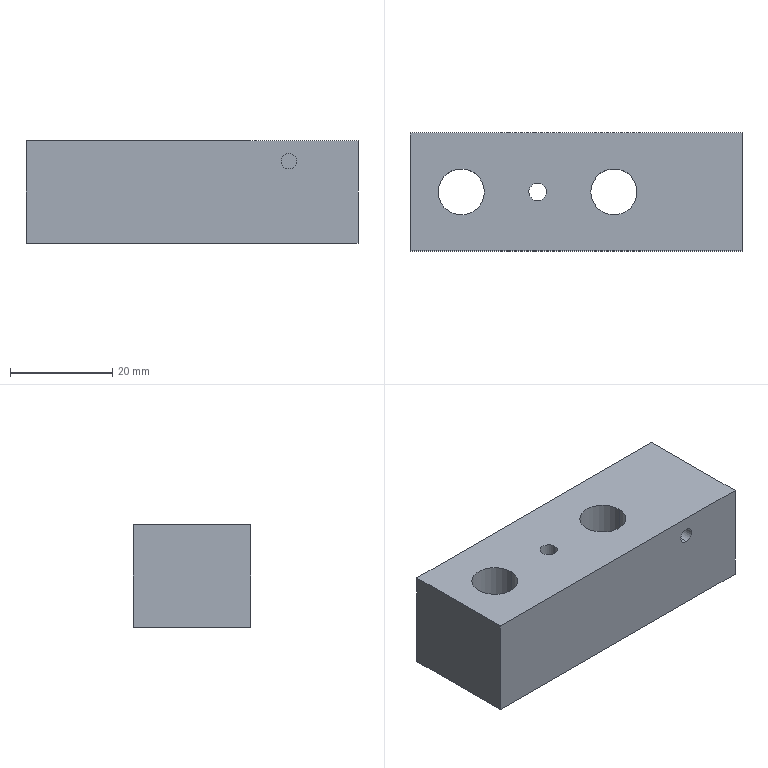Part | SolidWorks | features 3DProfileFeature 2, HoleWzd 2, Extrusion 1, ICE 1 | 1 solid | 24 faces | box 64.8 x 23 x 20 mm | volume 24913 mm3 | cylinder 14 | plane 10 | commonest cylinder face diameters 9 x4 15 x4 3 x2 3.4 x2 6.5 x2
STEP:
#1=CARTESIAN_POINT('',(-4.25,11.5,-6.6));
#2=VERTEX_POINT('',#1);
#3=CARTESIAN_POINT('',(-10.75,11.5,-6.6));
#4=VERTEX_POINT('',#3);
#5=CARTESIAN_POINT('',(-7.5,11.5,-6.6));
#6=DIRECTION('',(0.,0.,-1.));
#7=DIRECTION('',(-1.,0.,0.));
#8=AXIS2_PLACEMENT_3D('',#5,#6,#7);
#9=CIRCLE('',#8,3.25);
#10=EDGE_CURVE('',#2,#4,#9,.T.);
#11=ORIENTED_EDGE('',*,*,#10,.F.);
#12=CARTESIAN_POINT('',(-4.25,11.5,-10.));
#13=VERTEX_POINT('',#12);
#14=CARTESIAN_POINT('',(-4.25,11.5,-10.));
#15=DIRECTION('',(0.,0.,-1.));
#16=VECTOR('',#15,1000.);
#17=LINE('',#14,#16);
#18=EDGE_CURVE('',#2,#13,#17,.T.);
#19=ORIENTED_EDGE('',*,*,#18,.T.);
#20=CARTESIAN_POINT('',(-10.75,11.5,-10.));
#21=VERTEX_POINT('',#20);
#22=CARTESIAN_POINT('',(-7.5,11.5,-10.));
#23=DIRECTION('',(0.,0.,-1.));
#24=DIRECTION('',(-1.,0.,0.));
#25=AXIS2_PLACEMENT_3D('',#22,#23,#24);
#26=CIRCLE('',#25,3.25);
#27=EDGE_CURVE('',#13,#21,#26,.T.);
#28=ORIENTED_EDGE('',*,*,#27,.T.);
#29=CARTESIAN_POINT('',(-10.75,11.5,-10.));
#30=DIRECTION('',(0.,0.,-1.));
#31=VECTOR('',#30,1000.);
#32=LINE('',#29,#31);
#33=EDGE_CURVE('',#4,#21,#32,.T.);
#34=ORIENTED_EDGE('',*,*,#33,.F.);
#35=EDGE_LOOP('',(#11,#19,#28,#34));
#36=FACE_OUTER_BOUND('',#35,.T.);
#37=CARTESIAN_POINT('',(-7.5,11.5,-10.));
#38=DIRECTION('',(0.,0.,-1.));
#39=DIRECTION('',(-1.,0.,0.));
#40=AXIS2_PLACEMENT_3D('',#37,#38,#39);
#41=CYLINDRICAL_SURFACE('',#40,3.25);
#42=ADVANCED_FACE('',(#36),#41,.F.);
#43=CARTESIAN_POINT('',(-5.8,11.5,10.));
#44=VERTEX_POINT('',#43);
#45=CARTESIAN_POINT('',(-9.2,11.5,10.));
#46=VERTEX_POINT('',#45);
#47=CARTESIAN_POINT('',(-7.5,11.5,10.));
#48=DIRECTION('',(0.,0.,-1.));
#49=DIRECTION('',(-1.,0.,0.));
#50=AXIS2_PLACEMENT_3D('',#47,#48,#49);
#51=CIRCLE('',#50,1.7);
#52=EDGE_CURVE('',#44,#46,#51,.T.);
#53=ORIENTED_EDGE('',*,*,#52,.F.);
#54=CARTESIAN_POINT('',(-5.8,11.5,-6.6));
#55=VERTEX_POINT('',#54);
#56=CARTESIAN_POINT('',(-5.8,11.5,-10.));
#57=DIRECTION('',(0.,0.,-1.));
#58=VECTOR('',#57,1000.);
#59=LINE('',#56,#58);
#60=EDGE_CURVE('',#44,#55,#59,.T.);
#61=ORIENTED_EDGE('',*,*,#60,.T.);
#62=CARTESIAN_POINT('',(-9.2,11.5,-6.6));
#63=VERTEX_POINT('',#62);
#64=CARTESIAN_POINT('',(-7.5,11.5,-6.6));
#65=DIRECTION('',(0.,0.,-1.));
#66=DIRECTION('',(-1.,0.,0.));
#67=AXIS2_PLACEMENT_3D('',#64,#65,#66);
#68=CIRCLE('',#67,1.7);
#69=EDGE_CURVE('',#55,#63,#68,.T.);
#70=ORIENTED_EDGE('',*,*,#69,.T.);
#71=CARTESIAN_POINT('',(-9.2,11.5,-10.));
#72=DIRECTION('',(0.,0.,-1.));
#73=VECTOR('',#72,1000.);
#74=LINE('',#71,#73);
#75=EDGE_CURVE('',#46,#63,#74,.T.);
#76=ORIENTED_EDGE('',*,*,#75,.F.);
#77=EDGE_LOOP('',(#53,#61,#70,#76));
#78=FACE_OUTER_BOUND('',#77,.T.);
#79=CARTESIAN_POINT('',(-7.5,11.5,-10.));
#80=DIRECTION('',(0.,0.,-1.));
#81=DIRECTION('',(-1.,0.,0.));
#82=AXIS2_PLACEMENT_3D('',#79,#80,#81);
#83=CYLINDRICAL_SURFACE('',#82,1.7);
#84=ADVANCED_FACE('',(#78),#83,.F.);
#85=CARTESIAN_POINT('',(-14.9,11.5,-1.4));
#86=VERTEX_POINT('',#85);
#87=CARTESIAN_POINT('',(-29.9,11.5,-1.4));
#88=VERTEX_POINT('',#87);
#89=CARTESIAN_POINT('',(-22.4,11.5,-1.4));
#90=DIRECTION('',(0.,0.,-1.));
#91=DIRECTION('',(-1.,0.,0.));
#92=AXIS2_PLACEMENT_3D('',#89,#90,#91);
#93=CIRCLE('',#92,7.5);
#94=EDGE_CURVE('',#86,#88,#93,.T.);
#95=ORIENTED_EDGE('',*,*,#94,.F.);
#96=CARTESIAN_POINT('',(-14.9,11.5,-10.));
#97=VERTEX_POINT('',#96);
#98=CARTESIAN_POINT('',(-14.9,11.5,-10.));
#99=DIRECTION('',(0.,0.,-1.));
#100=VECTOR('',#99,1000.);
#101=LINE('',#98,#100);
#102=EDGE_CURVE('',#86,#97,#101,.T.);
#103=ORIENTED_EDGE('',*,*,#102,.T.);
#104=CARTESIAN_POINT('',(-29.9,11.5,-10.));
#105=VERTEX_POINT('',#104);
#106=CARTESIAN_POINT('',(-22.4,11.5,-10.));
#107=DIRECTION('',(0.,0.,-1.));
#108=DIRECTION('',(-1.,0.,0.));
#109=AXIS2_PLACEMENT_3D('',#106,#107,#108);
#110=CIRCLE('',#109,7.5);
#111=EDGE_CURVE('',#97,#105,#110,.T.);
#112=ORIENTED_EDGE('',*,*,#111,.T.);
#113=CARTESIAN_POINT('',(-29.9,11.5,-10.));
#114=DIRECTION('',(0.,0.,-1.));
#115=VECTOR('',#114,1000.);
#116=LINE('',#113,#115);
#117=EDGE_CURVE('',#88,#105,#116,.T.);
#118=ORIENTED_EDGE('',*,*,#117,.F.);
#119=EDGE_LOOP('',(#95,#103,#112,#118));
#120=FACE_OUTER_BOUND('',#119,.T.);
#121=CARTESIAN_POINT('',(-22.4,11.5,-10.));
#122=DIRECTION('',(0.,0.,-1.));
#123=DIRECTION('',(-1.,0.,0.));
#124=AXIS2_PLACEMENT_3D('',#121,#122,#123);
#125=CYLINDRICAL_SURFACE('',#124,7.5);
#126=ADVANCED_FACE('',(#120),#125,.F.);
#127=CARTESIAN_POINT('',(-17.9,11.5,10.));
#128=VERTEX_POINT('',#127);
#129=CARTESIAN_POINT('',(-26.9,11.5,10.));
#130=VERTEX_POINT('',#129);
#131=CARTESIAN_POINT('',(-22.4,11.5,10.));
#132=DIRECTION('',(0.,0.,-1.));
#133=DIRECTION('',(-1.,0.,0.));
#134=AXIS2_PLACEMENT_3D('',#131,#132,#133);
#135=CIRCLE('',#134,4.5);
#136=EDGE_CURVE('',#128,#130,#135,.T.);
#137=ORIENTED_EDGE('',*,*,#136,.F.);
#138=CARTESIAN_POINT('',(-17.9,11.5,-1.4));
#139=VERTEX_POINT('',#138);
#140=CARTESIAN_POINT('',(-17.9,11.5,-10.));
#141=DIRECTION('',(0.,0.,-1.));
#142=VECTOR('',#141,1000.);
#143=LINE('',#140,#142);
#144=EDGE_CURVE('',#128,#139,#143,.T.);
#145=ORIENTED_EDGE('',*,*,#144,.T.);
#146=CARTESIAN_POINT('',(-26.9,11.5,-1.4));
#147=VERTEX_POINT('',#146);
#148=CARTESIAN_POINT('',(-22.4,11.5,-1.4));
#149=DIRECTION('',(0.,0.,-1.));
#150=DIRECTION('',(-1.,0.,0.));
#151=AXIS2_PLACEMENT_3D('',#148,#149,#150);
#152=CIRCLE('',#151,4.5);
#153=EDGE_CURVE('',#139,#147,#152,.T.);
#154=ORIENTED_EDGE('',*,*,#153,.T.);
#155=CARTESIAN_POINT('',(-26.9,11.5,-10.));
#156=DIRECTION('',(0.,0.,-1.));
#157=VECTOR('',#156,1000.);
#158=LINE('',#155,#157);
#159=EDGE_CURVE('',#130,#147,#158,.T.);
#160=ORIENTED_EDGE('',*,*,#159,.F.);
#161=EDGE_LOOP('',(#137,#145,#154,#160));
#162=FACE_OUTER_BOUND('',#161,.T.);
#163=CARTESIAN_POINT('',(-22.4,11.5,-10.));
#164=DIRECTION('',(0.,0.,-1.));
#165=DIRECTION('',(-1.,0.,0.));
#166=AXIS2_PLACEMENT_3D('',#163,#164,#165);
#167=CYLINDRICAL_SURFACE('',#166,4.5);
#168=ADVANCED_FACE('',(#162),#167,.F.);
#169=CARTESIAN_POINT('',(14.9,11.5,-1.4));
#170=VERTEX_POINT('',#169);
#171=CARTESIAN_POINT('',(-0.1,11.5,-1.4));
#172=VERTEX_POINT('',#171);
#173=CARTESIAN_POINT('',(7.4,11.5,-1.4));
#174=DIRECTION('',(0.,0.,-1.));
#175=DIRECTION('',(-1.,0.,0.));
#176=AXIS2_PLACEMENT_3D('',#173,#174,#175);
#177=CIRCLE('',#176,7.5);
#178=EDGE_CURVE('',#170,#172,#177,.T.);
#179=ORIENTED_EDGE('',*,*,#178,.F.);
#180=CARTESIAN_POINT('',(14.9,11.5,-10.));
#181=VERTEX_POINT('',#180);
#182=CARTESIAN_POINT('',(14.9,11.5,-10.));
#183=DIRECTION('',(0.,0.,-1.));
#184=VECTOR('',#183,1000.);
#185=LINE('',#182,#184);
#186=EDGE_CURVE('',#170,#181,#185,.T.);
#187=ORIENTED_EDGE('',*,*,#186,.T.);
#188=CARTESIAN_POINT('',(-0.1,11.5,-10.));
#189=VERTEX_POINT('',#188);
#190=CARTESIAN_POINT('',(7.4,11.5,-10.));
#191=DIRECTION('',(0.,0.,-1.));
#192=DIRECTION('',(-1.,0.,0.));
#193=AXIS2_PLACEMENT_3D('',#190,#191,#192);
#194=CIRCLE('',#193,7.5);
#195=EDGE_CURVE('',#181,#189,#194,.T.);
#196=ORIENTED_EDGE('',*,*,#195,.T.);
#197=CARTESIAN_POINT('',(-0.1,11.5,-10.));
#198=DIRECTION('',(0.,0.,-1.));
#199=VECTOR('',#198,1000.);
#200=LINE('',#197,#199);
#201=EDGE_CURVE('',#172,#189,#200,.T.);
#202=ORIENTED_EDGE('',*,*,#201,.F.);
#203=EDGE_LOOP('',(#179,#187,#196,#202));
#204=FACE_OUTER_BOUND('',#203,.T.);
#205=CARTESIAN_POINT('',(7.4,11.5,-10.));
#206=DIRECTION('',(0.,0.,-1.));
#207=DIRECTION('',(-1.,0.,0.));
#208=AXIS2_PLACEMENT_3D('',#205,#206,#207);
#209=CYLINDRICAL_SURFACE('',#208,7.5);
#210=ADVANCED_FACE('',(#204),#209,.F.);
#211=CARTESIAN_POINT('',(11.9,11.5,10.));
#212=VERTEX_POINT('',#211);
#213=CARTESIAN_POINT('',(2.9,11.5,10.));
#214=VERTEX_POINT('',#213);
#215=CARTESIAN_POINT('',(7.4,11.5,10.));
#216=DIRECTION('',(0.,0.,-1.));
#217=DIRECTION('',(-1.,0.,0.));
#218=AXIS2_PLACEMENT_3D('',#215,#216,#217);
#219=CIRCLE('',#218,4.5);
#220=EDGE_CURVE('',#212,#214,#219,.T.);
#221=ORIENTED_EDGE('',*,*,#220,.F.);
#222=CARTESIAN_POINT('',(11.9,11.5,-1.4));
#223=VERTEX_POINT('',#222);
#224=CARTESIAN_POINT('',(11.9,11.5,-10.));
#225=DIRECTION('',(0.,0.,-1.));
#226=VECTOR('',#225,1000.);
#227=LINE('',#224,#226);
#228=EDGE_CURVE('',#212,#223,#227,.T.);
#229=ORIENTED_EDGE('',*,*,#228,.T.);
#230=CARTESIAN_POINT('',(2.9,11.5,-1.4));
#231=VERTEX_POINT('',#230);
#232=CARTESIAN_POINT('',(7.4,11.5,-1.4));
#233=DIRECTION('',(0.,0.,-1.));
#234=DIRECTION('',(-1.,0.,0.));
#235=AXIS2_PLACEMENT_3D('',#232,#233,#234);
#236=CIRCLE('',#235,4.5);
#237=EDGE_CURVE('',#223,#231,#236,.T.);
#238=ORIENTED_EDGE('',*,*,#237,.T.);
#239=CARTESIAN_POINT('',(2.9,11.5,-10.));
#240=DIRECTION('',(0.,0.,-1.));
#241=VECTOR('',#240,1000.);
#242=LINE('',#239,#241);
#243=EDGE_CURVE('',#214,#231,#242,.T.);
#244=ORIENTED_EDGE('',*,*,#243,.F.);
#245=EDGE_LOOP('',(#221,#229,#238,#244));
#246=FACE_OUTER_BOUND('',#245,.T.);
#247=CARTESIAN_POINT('',(7.4,11.5,-10.));
#248=DIRECTION('',(0.,0.,-1.));
#249=DIRECTION('',(-1.,0.,0.));
#250=AXIS2_PLACEMENT_3D('',#247,#248,#249);
#251=CYLINDRICAL_SURFACE('',#250,4.5);
#252=ADVANCED_FACE('',(#246),#251,.F.);
#253=CARTESIAN_POINT('',(18.9,20.,4.5));
#254=VERTEX_POINT('',#253);
#255=CARTESIAN_POINT('',(18.9,20.,7.5));
#256=VERTEX_POINT('',#255);
#257=CARTESIAN_POINT('',(18.9,20.,6.));
#258=DIRECTION('',(0.,1.,0.));
#259=DIRECTION('',(0.,0.,1.));
#260=AXIS2_PLACEMENT_3D('',#257,#258,#259);
#261=CIRCLE('',#260,1.5);
#262=EDGE_CURVE('',#254,#256,#261,.T.);
#263=ORIENTED_EDGE('',*,*,#262,.T.);
#264=CARTESIAN_POINT('',(18.9,0.,7.5));
#265=VERTEX_POINT('',#264);
#266=CARTESIAN_POINT('',(18.9,20.,7.5));
#267=DIRECTION('',(0.,-1.,0.));
#268=VECTOR('',#267,1000.);
#269=LINE('',#266,#268);
#270=EDGE_CURVE('',#256,#265,#269,.T.);
#271=ORIENTED_EDGE('',*,*,#270,.T.);
#272=CARTESIAN_POINT('',(18.9,0.,4.5));
#273=VERTEX_POINT('',#272);
#274=CARTESIAN_POINT('',(18.9,0.,6.));
#275=DIRECTION('',(0.,1.,0.));
#276=DIRECTION('',(0.,0.,1.));
#277=AXIS2_PLACEMENT_3D('',#274,#275,#276);
#278=CIRCLE('',#277,1.5);
#279=EDGE_CURVE('',#273,#265,#278,.T.);
#280=ORIENTED_EDGE('',*,*,#279,.F.);
#281=CARTESIAN_POINT('',(18.9,20.,4.5));
#282=DIRECTION('',(0.,-1.,0.));
#283=VECTOR('',#282,1000.);
#284=LINE('',#281,#283);
#285=EDGE_CURVE('',#254,#273,#284,.T.);
#286=ORIENTED_EDGE('',*,*,#285,.F.);
#287=EDGE_LOOP('',(#263,#271,#280,#286));
#288=FACE_OUTER_BOUND('',#287,.T.);
#289=CARTESIAN_POINT('',(18.9,20.,6.));
#290=DIRECTION('',(0.,-1.,0.));
#291=DIRECTION('',(0.,0.,-1.));
#292=AXIS2_PLACEMENT_3D('',#289,#290,#291);
#293=CYLINDRICAL_SURFACE('',#292,1.5);
#294=ADVANCED_FACE('',(#288),#293,.F.);
#295=CARTESIAN_POINT('',(-32.4,0.,-10.));
#296=VERTEX_POINT('',#295);
#297=CARTESIAN_POINT('',(-32.4,0.,10.));
#298=VERTEX_POINT('',#297);
#299=CARTESIAN_POINT('',(-32.4,0.,-10.));
#300=DIRECTION('',(0.,0.,1.));
#301=VECTOR('',#300,1000.);
#302=LINE('',#299,#301);
#303=EDGE_CURVE('',#296,#298,#302,.T.);
#304=ORIENTED_EDGE('',*,*,#303,.T.);
#305=CARTESIAN_POINT('',(-32.4,23.,10.));
#306=VERTEX_POINT('',#305);
#307=CARTESIAN_POINT('',(-32.4,23.,10.));
#308=DIRECTION('',(0.,-1.,0.));
#309=VECTOR('',#308,1000.);
#310=LINE('',#307,#309);
#311=EDGE_CURVE('',#306,#298,#310,.T.);
#312=ORIENTED_EDGE('',*,*,#311,.F.);
#313=CARTESIAN_POINT('',(-32.4,23.,-10.));
#314=VERTEX_POINT('',#313);
#315=CARTESIAN_POINT('',(-32.4,23.,-10.));
#316=DIRECTION('',(0.,0.,1.));
#317=VECTOR('',#316,1000.);
#318=LINE('',#315,#317);
#319=EDGE_CURVE('',#314,#306,#318,.T.);
#320=ORIENTED_EDGE('',*,*,#319,.F.);
#321=CARTESIAN_POINT('',(-32.4,23.,-10.));
#322=DIRECTION('',(0.,-1.,0.));
#323=VECTOR('',#322,1000.);
#324=LINE('',#321,#323);
#325=EDGE_CURVE('',#314,#296,#324,.T.);
#326=ORIENTED_EDGE('',*,*,#325,.T.);
#327=EDGE_LOOP('',(#304,#312,#320,#326));
#328=FACE_OUTER_BOUND('',#327,.T.);
#329=CARTESIAN_POINT('',(-32.4,23.,-10.));
#330=DIRECTION('',(1.,0.,0.));
#331=DIRECTION('',(0.,0.,-1.));
#332=AXIS2_PLACEMENT_3D('',#329,#330,#331);
#333=PLANE('',#332);
#334=ADVANCED_FACE('',(#328),#333,.F.);
#335=CARTESIAN_POINT('',(-7.5,11.5,10.));
#336=DIRECTION('',(0.,0.,-1.));
#337=DIRECTION('',(-1.,0.,0.));
#338=AXIS2_PLACEMENT_3D('',#335,#336,#337);
#339=CIRCLE('',#338,1.7);
#340=EDGE_CURVE('',#46,#44,#339,.T.);
#341=ORIENTED_EDGE('',*,*,#340,.T.);
#342=ORIENTED_EDGE('',*,*,#52,.T.);
#343=EDGE_LOOP('',(#341,#342));
#344=FACE_BOUND('',#343,.T.);
#345=CARTESIAN_POINT('',(-22.4,11.5,10.));
#346=DIRECTION('',(0.,0.,-1.));
#347=DIRECTION('',(-1.,0.,0.));
#348=AXIS2_PLACEMENT_3D('',#345,#346,#347);
#349=CIRCLE('',#348,4.5);
#350=EDGE_CURVE('',#130,#128,#349,.T.);
#351=ORIENTED_EDGE('',*,*,#350,.T.);
#352=ORIENTED_EDGE('',*,*,#136,.T.);
#353=EDGE_LOOP('',(#351,#352));
#354=FACE_BOUND('',#353,.T.);
#355=CARTESIAN_POINT('',(7.4,11.5,10.));
#356=DIRECTION('',(0.,0.,-1.));
#357=DIRECTION('',(-1.,0.,0.));
#358=AXIS2_PLACEMENT_3D('',#355,#356,#357);
#359=CIRCLE('',#358,4.5);
#360=EDGE_CURVE('',#214,#212,#359,.T.);
#361=ORIENTED_EDGE('',*,*,#360,.T.);
#362=ORIENTED_EDGE('',*,*,#220,.T.);
#363=EDGE_LOOP('',(#361,#362));
#364=FACE_BOUND('',#363,.T.);
#365=CARTESIAN_POINT('',(32.4,0.,10.));
#366=VERTEX_POINT('',#365);
#367=CARTESIAN_POINT('',(32.4,0.,10.));
#368=DIRECTION('',(1.,0.,0.));
#369=VECTOR('',#368,1000.);
#370=LINE('',#367,#369);
#371=EDGE_CURVE('',#298,#366,#370,.T.);
#372=ORIENTED_EDGE('',*,*,#371,.T.);
#373=CARTESIAN_POINT('',(32.4,23.,10.));
#374=VERTEX_POINT('',#373);
#375=CARTESIAN_POINT('',(32.4,23.,10.));
#376=DIRECTION('',(0.,-1.,0.));
#377=VECTOR('',#376,1000.);
#378=LINE('',#375,#377);
#379=EDGE_CURVE('',#374,#366,#378,.T.);
#380=ORIENTED_EDGE('',*,*,#379,.F.);
#381=CARTESIAN_POINT('',(32.4,23.,10.));
#382=DIRECTION('',(1.,0.,0.));
#383=VECTOR('',#382,1000.);
#384=LINE('',#381,#383);
#385=EDGE_CURVE('',#306,#374,#384,.T.);
#386=ORIENTED_EDGE('',*,*,#385,.F.);
#387=ORIENTED_EDGE('',*,*,#311,.T.);
#388=EDGE_LOOP('',(#372,#380,#386,#387));
#389=FACE_OUTER_BOUND('',#388,.T.);
#390=CARTESIAN_POINT('',(32.4,23.,10.));
#391=DIRECTION('',(0.,0.,-1.));
#392=DIRECTION('',(-1.,0.,0.));
#393=AXIS2_PLACEMENT_3D('',#390,#391,#392);
#394=PLANE('',#393);
#395=ADVANCED_FACE('',(#344,#354,#364,#389),#394,.F.);
#396=CARTESIAN_POINT('',(32.4,0.,-10.));
#397=VERTEX_POINT('',#396);
#398=CARTESIAN_POINT('',(32.4,0.,-10.));
#399=DIRECTION('',(0.,0.,-1.));
#400=VECTOR('',#399,1000.);
#401=LINE('',#398,#400);
#402=EDGE_CURVE('',#366,#397,#401,.T.);
#403=ORIENTED_EDGE('',*,*,#402,.T.);
#404=CARTESIAN_POINT('',(32.4,23.,-10.));
#405=VERTEX_POINT('',#404);
#406=CARTESIAN_POINT('',(32.4,23.,-10.));
#407=DIRECTION('',(0.,-1.,0.));
#408=VECTOR('',#407,1000.);
#409=LINE('',#406,#408);
#410=EDGE_CURVE('',#405,#397,#409,.T.);
#411=ORIENTED_EDGE('',*,*,#410,.F.);
#412=CARTESIAN_POINT('',(32.4,23.,-10.));
#413=DIRECTION('',(0.,0.,-1.));
#414=VECTOR('',#413,1000.);
#415=LINE('',#412,#414);
#416=EDGE_CURVE('',#374,#405,#415,.T.);
#417=ORIENTED_EDGE('',*,*,#416,.F.);
#418=ORIENTED_EDGE('',*,*,#379,.T.);
#419=EDGE_LOOP('',(#403,#411,#417,#418));
#420=FACE_OUTER_BOUND('',#419,.T.);
#421=CARTESIAN_POINT('',(32.4,23.,-10.));
#422=DIRECTION('',(-1.,0.,0.));
#423=DIRECTION('',(0.,0.,1.));
#424=AXIS2_PLACEMENT_3D('',#421,#422,#423);
#425=PLANE('',#424);
#426=ADVANCED_FACE('',(#420),#425,.F.);
#427=CARTESIAN_POINT('',(-7.5,11.5,-10.));
#428=DIRECTION('',(0.,0.,-1.));
#429=DIRECTION('',(-1.,0.,0.));
#430=AXIS2_PLACEMENT_3D('',#427,#428,#429);
#431=CIRCLE('',#430,3.25);
#432=EDGE_CURVE('',#21,#13,#431,.T.);
#433=ORIENTED_EDGE('',*,*,#432,.F.);
#434=ORIENTED_EDGE('',*,*,#27,.F.);
#435=EDGE_LOOP('',(#433,#434));
#436=FACE_BOUND('',#435,.T.);
#437=CARTESIAN_POINT('',(-22.4,11.5,-10.));
#438=DIRECTION('',(0.,0.,-1.));
#439=DIRECTION('',(-1.,0.,0.));
#440=AXIS2_PLACEMENT_3D('',#437,#438,#439);
#441=CIRCLE('',#440,7.5);
#442=EDGE_CURVE('',#105,#97,#441,.T.);
#443=ORIENTED_EDGE('',*,*,#442,.F.);
#444=ORIENTED_EDGE('',*,*,#111,.F.);
#445=EDGE_LOOP('',(#443,#444));
#446=FACE_BOUND('',#445,.T.);
#447=CARTESIAN_POINT('',(7.4,11.5,-10.));
#448=DIRECTION('',(0.,0.,-1.));
#449=DIRECTION('',(-1.,0.,0.));
#450=AXIS2_PLACEMENT_3D('',#447,#448,#449);
#451=CIRCLE('',#450,7.5);
#452=EDGE_CURVE('',#189,#181,#451,.T.);
#453=ORIENTED_EDGE('',*,*,#452,.F.);
#454=ORIENTED_EDGE('',*,*,#195,.F.);
#455=EDGE_LOOP('',(#453,#454));
#456=FACE_BOUND('',#455,.T.);
#457=CARTESIAN_POINT('',(32.4,0.,-10.));
#458=DIRECTION('',(-1.,0.,0.));
#459=VECTOR('',#458,1000.);
#460=LINE('',#457,#459);
#461=EDGE_CURVE('',#397,#296,#460,.T.);
#462=ORIENTED_EDGE('',*,*,#461,.T.);
#463=ORIENTED_EDGE('',*,*,#325,.F.);
#464=CARTESIAN_POINT('',(32.4,23.,-10.));
#465=DIRECTION('',(-1.,0.,0.));
#466=VECTOR('',#465,1000.);
#467=LINE('',#464,#466);
#468=EDGE_CURVE('',#405,#314,#467,.T.);
#469=ORIENTED_EDGE('',*,*,#468,.F.);
#470=ORIENTED_EDGE('',*,*,#410,.T.);
#471=EDGE_LOOP('',(#462,#463,#469,#470));
#472=FACE_OUTER_BOUND('',#471,.T.);
#473=CARTESIAN_POINT('',(32.4,23.,-10.));
#474=DIRECTION('',(0.,0.,1.));
#475=DIRECTION('',(1.,0.,0.));
#476=AXIS2_PLACEMENT_3D('',#473,#474,#475);
#477=PLANE('',#476);
#478=ADVANCED_FACE('',(#436,#446,#456,#472),#477,.F.);
#479=ORIENTED_EDGE('',*,*,#319,.T.);
#480=ORIENTED_EDGE('',*,*,#385,.T.);
#481=ORIENTED_EDGE('',*,*,#416,.T.);
#482=ORIENTED_EDGE('',*,*,#468,.T.);
#483=EDGE_LOOP('',(#479,#480,#481,#482));
#484=FACE_OUTER_BOUND('',#483,.T.);
#485=CARTESIAN_POINT('',(0.,23.,0.));
#486=DIRECTION('',(0.,-1.,0.));
#487=DIRECTION('',(0.,0.,-1.));
#488=AXIS2_PLACEMENT_3D('',#485,#486,#487);
#489=PLANE('',#488);
#490=ADVANCED_FACE('',(#484),#489,.F.);
#491=ORIENTED_EDGE('',*,*,#279,.T.);
#492=CARTESIAN_POINT('',(18.9,0.,6.));
#493=DIRECTION('',(0.,1.,0.));
#494=DIRECTION('',(0.,0.,1.));
#495=AXIS2_PLACEMENT_3D('',#492,#493,#494);
#496=CIRCLE('',#495,1.5);
#497=EDGE_CURVE('',#265,#273,#496,.T.);
#498=ORIENTED_EDGE('',*,*,#497,.T.);
#499=EDGE_LOOP('',(#491,#498));
#500=FACE_BOUND('',#499,.T.);
#501=ORIENTED_EDGE('',*,*,#303,.F.);
#502=ORIENTED_EDGE('',*,*,#461,.F.);
#503=ORIENTED_EDGE('',*,*,#402,.F.);
#504=ORIENTED_EDGE('',*,*,#371,.F.);
#505=EDGE_LOOP('',(#501,#502,#503,#504));
#506=FACE_OUTER_BOUND('',#505,.T.);
#507=CARTESIAN_POINT('',(0.,0.,0.));
#508=DIRECTION('',(0.,-1.,0.));
#509=DIRECTION('',(0.,0.,-1.));
#510=AXIS2_PLACEMENT_3D('',#507,#508,#509);
#511=PLANE('',#510);
#512=ADVANCED_FACE('',(#500,#506),#511,.T.);
#513=ORIENTED_EDGE('',*,*,#270,.F.);
#514=CARTESIAN_POINT('',(18.9,20.,6.));
#515=DIRECTION('',(0.,1.,0.));
#516=DIRECTION('',(0.,0.,1.));
#517=AXIS2_PLACEMENT_3D('',#514,#515,#516);
#518=CIRCLE('',#517,1.5);
#519=EDGE_CURVE('',#256,#254,#518,.T.);
#520=ORIENTED_EDGE('',*,*,#519,.T.);
#521=ORIENTED_EDGE('',*,*,#285,.T.);
#522=ORIENTED_EDGE('',*,*,#497,.F.);
#523=EDGE_LOOP('',(#513,#520,#521,#522));
#524=FACE_OUTER_BOUND('',#523,.T.);
#525=CARTESIAN_POINT('',(18.9,20.,6.));
#526=DIRECTION('',(0.,-1.,0.));
#527=DIRECTION('',(0.,0.,-1.));
#528=AXIS2_PLACEMENT_3D('',#525,#526,#527);
#529=CYLINDRICAL_SURFACE('',#528,1.5);
#530=ADVANCED_FACE('',(#524),#529,.F.);
#531=ORIENTED_EDGE('',*,*,#262,.F.);
#532=ORIENTED_EDGE('',*,*,#519,.F.);
#533=EDGE_LOOP('',(#531,#532));
#534=FACE_OUTER_BOUND('',#533,.T.);
#535=CARTESIAN_POINT('',(18.9,20.,6.));
#536=DIRECTION('',(0.,1.,0.));
#537=DIRECTION('',(0.,0.,1.));
#538=AXIS2_PLACEMENT_3D('',#535,#536,#537);
#539=PLANE('',#538);
#540=ADVANCED_FACE('',(#534),#539,.F.);
#541=ORIENTED_EDGE('',*,*,#228,.F.);
#542=ORIENTED_EDGE('',*,*,#360,.F.);
#543=ORIENTED_EDGE('',*,*,#243,.T.);
#544=CARTESIAN_POINT('',(7.4,11.5,-1.4));
#545=DIRECTION('',(0.,0.,-1.));
#546=DIRECTION('',(-1.,0.,0.));
#547=AXIS2_PLACEMENT_3D('',#544,#545,#546);
#548=CIRCLE('',#547,4.5);
#549=EDGE_CURVE('',#231,#223,#548,.T.);
#550=ORIENTED_EDGE('',*,*,#549,.T.);
#551=EDGE_LOOP('',(#541,#542,#543,#550));
#552=FACE_OUTER_BOUND('',#551,.T.);
#553=CARTESIAN_POINT('',(7.4,11.5,-10.));
#554=DIRECTION('',(0.,0.,-1.));
#555=DIRECTION('',(-1.,0.,0.));
#556=AXIS2_PLACEMENT_3D('',#553,#554,#555);
#557=CYLINDRICAL_SURFACE('',#556,4.5);
#558=ADVANCED_FACE('',(#552),#557,.F.);
#559=ORIENTED_EDGE('',*,*,#549,.F.);
#560=ORIENTED_EDGE('',*,*,#237,.F.);
#561=EDGE_LOOP('',(#559,#560));
#562=FACE_BOUND('',#561,.T.);
#563=CARTESIAN_POINT('',(7.4,11.5,-1.4));
#564=DIRECTION('',(0.,0.,-1.));
#565=DIRECTION('',(-1.,0.,0.));
#566=AXIS2_PLACEMENT_3D('',#563,#564,#565);
#567=CIRCLE('',#566,7.5);
#568=EDGE_CURVE('',#172,#170,#567,.T.);
#569=ORIENTED_EDGE('',*,*,#568,.T.);
#570=ORIENTED_EDGE('',*,*,#178,.T.);
#571=EDGE_LOOP('',(#569,#570));
#572=FACE_OUTER_BOUND('',#571,.T.);
#573=CARTESIAN_POINT('',(11.9,11.5,-1.4));
#574=DIRECTION('',(0.,0.,1.));
#575=DIRECTION('',(1.,0.,0.));
#576=AXIS2_PLACEMENT_3D('',#573,#574,#575);
#577=PLANE('',#576);
#578=ADVANCED_FACE('',(#562,#572),#577,.F.);
#579=ORIENTED_EDGE('',*,*,#186,.F.);
#580=ORIENTED_EDGE('',*,*,#568,.F.);
#581=ORIENTED_EDGE('',*,*,#201,.T.);
#582=ORIENTED_EDGE('',*,*,#452,.T.);
#583=EDGE_LOOP('',(#579,#580,#581,#582));
#584=FACE_OUTER_BOUND('',#583,.T.);
#585=CARTESIAN_POINT('',(7.4,11.5,-10.));
#586=DIRECTION('',(0.,0.,-1.));
#587=DIRECTION('',(-1.,0.,0.));
#588=AXIS2_PLACEMENT_3D('',#585,#586,#587);
#589=CYLINDRICAL_SURFACE('',#588,7.5);
#590=ADVANCED_FACE('',(#584),#589,.F.);
#591=ORIENTED_EDGE('',*,*,#144,.F.);
#592=ORIENTED_EDGE('',*,*,#350,.F.);
#593=ORIENTED_EDGE('',*,*,#159,.T.);
#594=CARTESIAN_POINT('',(-22.4,11.5,-1.4));
#595=DIRECTION('',(0.,0.,-1.));
#596=DIRECTION('',(-1.,0.,0.));
#597=AXIS2_PLACEMENT_3D('',#594,#595,#596);
#598=CIRCLE('',#597,4.5);
#599=EDGE_CURVE('',#147,#139,#598,.T.);
#600=ORIENTED_EDGE('',*,*,#599,.T.);
#601=EDGE_LOOP('',(#591,#592,#593,#600));
#602=FACE_OUTER_BOUND('',#601,.T.);
#603=CARTESIAN_POINT('',(-22.4,11.5,-10.));
#604=DIRECTION('',(0.,0.,-1.));
#605=DIRECTION('',(-1.,0.,0.));
#606=AXIS2_PLACEMENT_3D('',#603,#604,#605);
#607=CYLINDRICAL_SURFACE('',#606,4.5);
#608=ADVANCED_FACE('',(#602),#607,.F.);
#609=ORIENTED_EDGE('',*,*,#599,.F.);
#610=ORIENTED_EDGE('',*,*,#153,.F.);
#611=EDGE_LOOP('',(#609,#610));
#612=FACE_BOUND('',#611,.T.);
#613=CARTESIAN_POINT('',(-22.4,11.5,-1.4));
#614=DIRECTION('',(0.,0.,-1.));
#615=DIRECTION('',(-1.,0.,0.));
#616=AXIS2_PLACEMENT_3D('',#613,#614,#615);
#617=CIRCLE('',#616,7.5);
#618=EDGE_CURVE('',#88,#86,#617,.T.);
#619=ORIENTED_EDGE('',*,*,#618,.T.);
#620=ORIENTED_EDGE('',*,*,#94,.T.);
#621=EDGE_LOOP('',(#619,#620));
#622=FACE_OUTER_BOUND('',#621,.T.);
#623=CARTESIAN_POINT('',(-17.9,11.5,-1.4));
#624=DIRECTION('',(0.,0.,1.));
#625=DIRECTION('',(1.,0.,0.));
#626=AXIS2_PLACEMENT_3D('',#623,#624,#625);
#627=PLANE('',#626);
#628=ADVANCED_FACE('',(#612,#622),#627,.F.);
#629=ORIENTED_EDGE('',*,*,#102,.F.);
#630=ORIENTED_EDGE('',*,*,#618,.F.);
#631=ORIENTED_EDGE('',*,*,#117,.T.);
#632=ORIENTED_EDGE('',*,*,#442,.T.);
#633=EDGE_LOOP('',(#629,#630,#631,#632));
#634=FACE_OUTER_BOUND('',#633,.T.);
#635=CARTESIAN_POINT('',(-22.4,11.5,-10.));
#636=DIRECTION('',(0.,0.,-1.));
#637=DIRECTION('',(-1.,0.,0.));
#638=AXIS2_PLACEMENT_3D('',#635,#636,#637);
#639=CYLINDRICAL_SURFACE('',#638,7.5);
#640=ADVANCED_FACE('',(#634),#639,.F.);
#641=ORIENTED_EDGE('',*,*,#60,.F.);
#642=ORIENTED_EDGE('',*,*,#340,.F.);
#643=ORIENTED_EDGE('',*,*,#75,.T.);
#644=CARTESIAN_POINT('',(-7.5,11.5,-6.6));
#645=DIRECTION('',(0.,0.,-1.));
#646=DIRECTION('',(-1.,0.,0.));
#647=AXIS2_PLACEMENT_3D('',#644,#645,#646);
#648=CIRCLE('',#647,1.7);
#649=EDGE_CURVE('',#63,#55,#648,.T.);
#650=ORIENTED_EDGE('',*,*,#649,.T.);
#651=EDGE_LOOP('',(#641,#642,#643,#650));
#652=FACE_OUTER_BOUND('',#651,.T.);
#653=CARTESIAN_POINT('',(-7.5,11.5,-10.));
#654=DIRECTION('',(0.,0.,-1.));
#655=DIRECTION('',(-1.,0.,0.));
#656=AXIS2_PLACEMENT_3D('',#653,#654,#655);
#657=CYLINDRICAL_SURFACE('',#656,1.7);
#658=ADVANCED_FACE('',(#652),#657,.F.);
#659=ORIENTED_EDGE('',*,*,#649,.F.);
#660=ORIENTED_EDGE('',*,*,#69,.F.);
#661=EDGE_LOOP('',(#659,#660));
#662=FACE_BOUND('',#661,.T.);
#663=CARTESIAN_POINT('',(-7.5,11.5,-6.6));
#664=DIRECTION('',(0.,0.,-1.));
#665=DIRECTION('',(-1.,0.,0.));
#666=AXIS2_PLACEMENT_3D('',#663,#664,#665);
#667=CIRCLE('',#666,3.25);
#668=EDGE_CURVE('',#4,#2,#667,.T.);
#669=ORIENTED_EDGE('',*,*,#668,.T.);
#670=ORIENTED_EDGE('',*,*,#10,.T.);
#671=EDGE_LOOP('',(#669,#670));
#672=FACE_OUTER_BOUND('',#671,.T.);
#673=CARTESIAN_POINT('',(-5.8,11.5,-6.6));
#674=DIRECTION('',(0.,0.,1.));
#675=DIRECTION('',(1.,0.,0.));
#676=AXIS2_PLACEMENT_3D('',#673,#674,#675);
#677=PLANE('',#676);
#678=ADVANCED_FACE('',(#662,#672),#677,.F.);
#679=ORIENTED_EDGE('',*,*,#18,.F.);
#680=ORIENTED_EDGE('',*,*,#668,.F.);
#681=ORIENTED_EDGE('',*,*,#33,.T.);
#682=ORIENTED_EDGE('',*,*,#432,.T.);
#683=EDGE_LOOP('',(#679,#680,#681,#682));
#684=FACE_OUTER_BOUND('',#683,.T.);
#685=CARTESIAN_POINT('',(-7.5,11.5,-10.));
#686=DIRECTION('',(0.,0.,-1.));
#687=DIRECTION('',(-1.,0.,0.));
#688=AXIS2_PLACEMENT_3D('',#685,#686,#687);
#689=CYLINDRICAL_SURFACE('',#688,3.25);
#690=ADVANCED_FACE('',(#684),#689,.F.);
#691=CLOSED_SHELL('',(#42,#84,#126,#168,#210,#252,#294,#334,#395,#426,#478,#490,#512,#530,#540,#558,#578,#590,#608,#628,#640,#658,#678,#690));
#692=MANIFOLD_SOLID_BREP('',#691);
#693=CARTESIAN_POINT('',(0.,0.,0.));
#694=DIRECTION('',(0.,0.,1.));
#695=DIRECTION('',(1.,0.,0.));
#696=AXIS2_PLACEMENT_3D('',#693,#694,#695);
#697=(LENGTH_UNIT()NAMED_UNIT(*)SI_UNIT(.MILLI.,.METRE.));
#698=UNCERTAINTY_MEASURE_WITH_UNIT(LENGTH_MEASURE(0.00001),#697,'','');
#699=(NAMED_UNIT(*)PLANE_ANGLE_UNIT()SI_UNIT($,.RADIAN.));
#700=(NAMED_UNIT(*)SI_UNIT($,.STERADIAN.)SOLID_ANGLE_UNIT());
#701=(GEOMETRIC_REPRESENTATION_CONTEXT(3)GLOBAL_UNCERTAINTY_ASSIGNED_CONTEXT((#698))GLOBAL_UNIT_ASSIGNED_CONTEXT((#697,#699,#700))REPRESENTATION_CONTEXT('',''));
#702=ADVANCED_BREP_SHAPE_REPRESENTATION('',(#692,#696),#701);